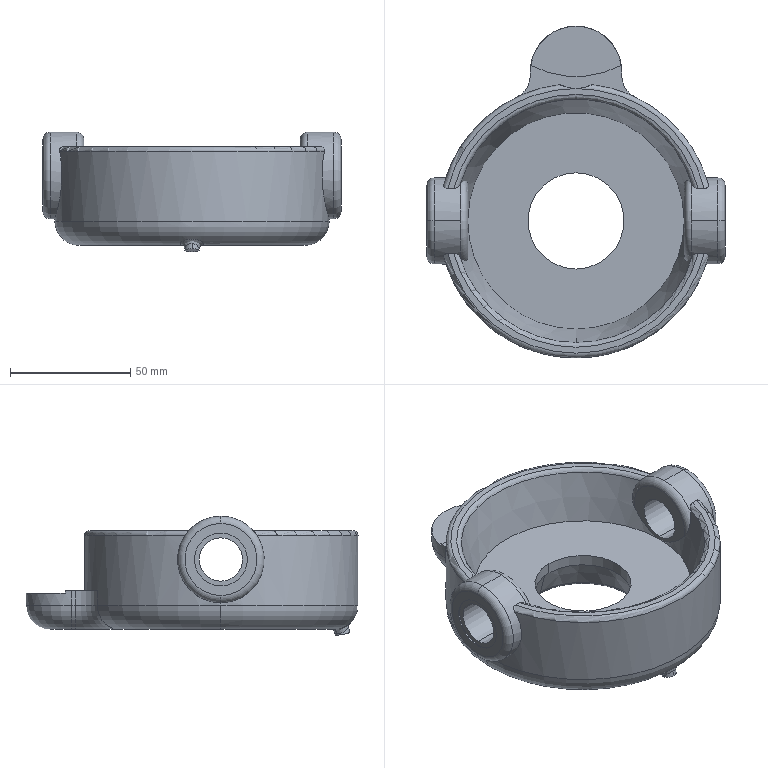Part | SolidWorks | features ICE 6, Fillet 5, Extrusion 1, HoleWzd 1, MirrorPattern 1, RevCut 1, Sculpt 1, Sweep 1 | 1 solid | 75 faces | box 124 x 138 x 49.724 mm | volume 237420 mm3 | cylinder 28 | torus 19 | plane 16 | cone 9 | spline 3 | commonest cylinder face diameters 18 x4 20 x4 22 x4 36 x4 114 x3 3 x2